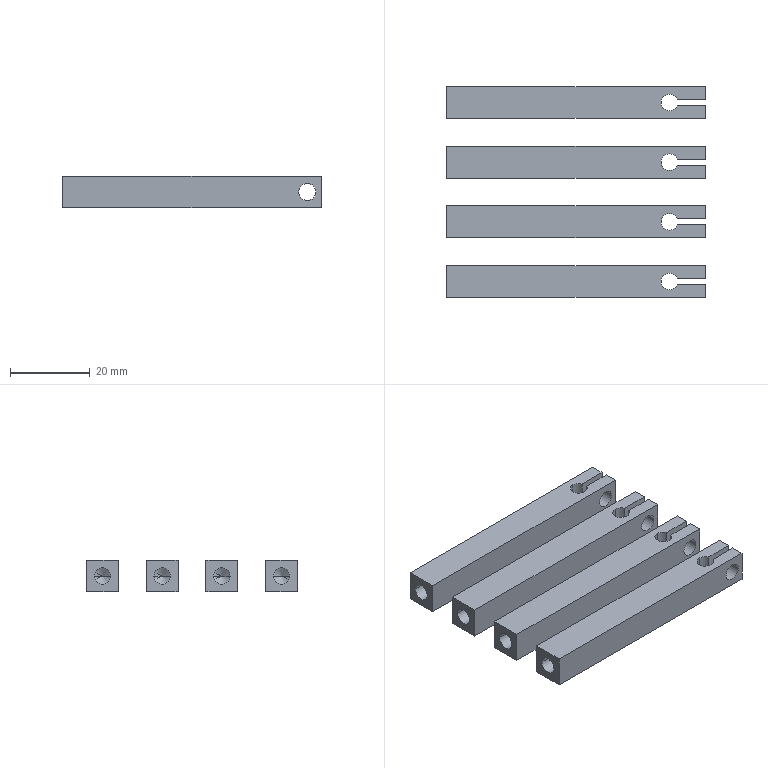NC program | NX | posted with a generic post | part box 65 x 53 x 8 mm
Whole program:
N10 G17 G21 G94 G90
(DRILLING_COPY_COPY_1 , TOOL : D6A45)
N12 T07 M6
N14 G54
N16 G17 G0 G90 X0. Y0. B0. C0. S5000 M3
N18 G43 Z30. H7
N20 G94 G81 G98 Z-2.25 F250. R3.
N22 G80
N24 G0 X0. Y0. Z30.
N26 M5
(DRILLING_COPY_COPY_COPY_1 , TOOL : 4.2ZT)
N28 T14 M6
N30 G54
N32 G17 G0 G90 X0. Y0. B0. C0. S2000 M3
N34 G43 Z30. H14
N36 G94 G83 G98 Z-13.662 F200. Q2. R3.
N38 G80
N40 G0 X0. Y0. Z30.
N42 M5
N44 M2